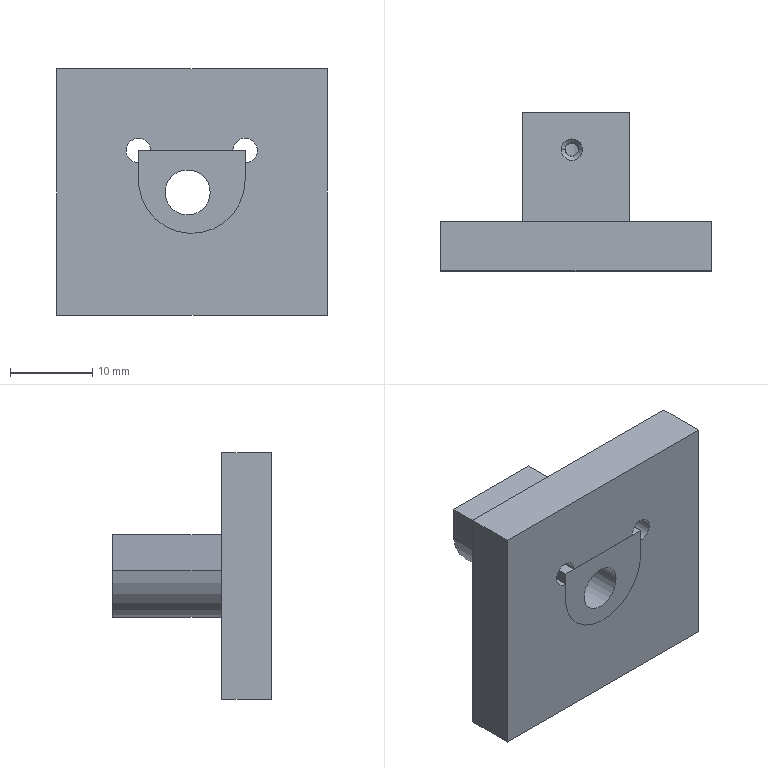NC program | NX | posted with a generic post | part box 32.951 x 19.3 x 30.1 mm
Whole program:
N10 G17 G21 G94 G90
(DRILLING , TOOL : D6A45)
N12 T07 M6
N14 G54
N16 G17 G0 G90 X-5.51 Y0.5 B0. C0. S5000 M3
N18 G43 Z30. H7
N20 G94 G81 G98 Z-1.3 F250. R3.
N22 X5.15
N24 G80
N26 G0 X5.15 Y0.5 Z30.
N28 M5
(DRILLING_COPY , TOOL : 1.6ZT)
N30 T16 M6
N32 G54
N34 G17 G0 G90 X-5.51 Y0.5 B0. C0. S2000 M3
N36 G43 Z30. H16
N38 G94 G83 G98 Z-4.45 F100. Q2. R3.
N40 X5.15
N42 G80
N44 G0 X5.15 Y0.5 Z30.
N46 M5
(PLANAR_MILL , TOOL : D6A45)
N48 T07 M6
N50 G54
N52 G17 G0 G90 X-1.473 Y8.6 B0. C0. S9500 M3
N54 G43 Z30. H7
N56 Z0.5
N58 G94 G1 Z-1. F1250.
N60 X-0.766 Y7.757
N62 G3 X0. Y7.4 R1.
N64 G1 X9.55
N66 G2 X10.55 Y6.4 R1.
N68 G1 Y-6.4
N70 G2 X9.55 Y-7.4 R1.
N72 G1 X-9.55
N74 G2 X-10.55 Y-6.4 R1.
N76 G1 Y6.4
N78 G2 X-9.55 Y7.4 R1.
N80 G1 X0.
N82 G3 X0.766 Y7.757 R1.
N84 G1 X1.473 Y8.6
N86 Z0.5
N88 G0 Z30.
N90 M5
N92 M2